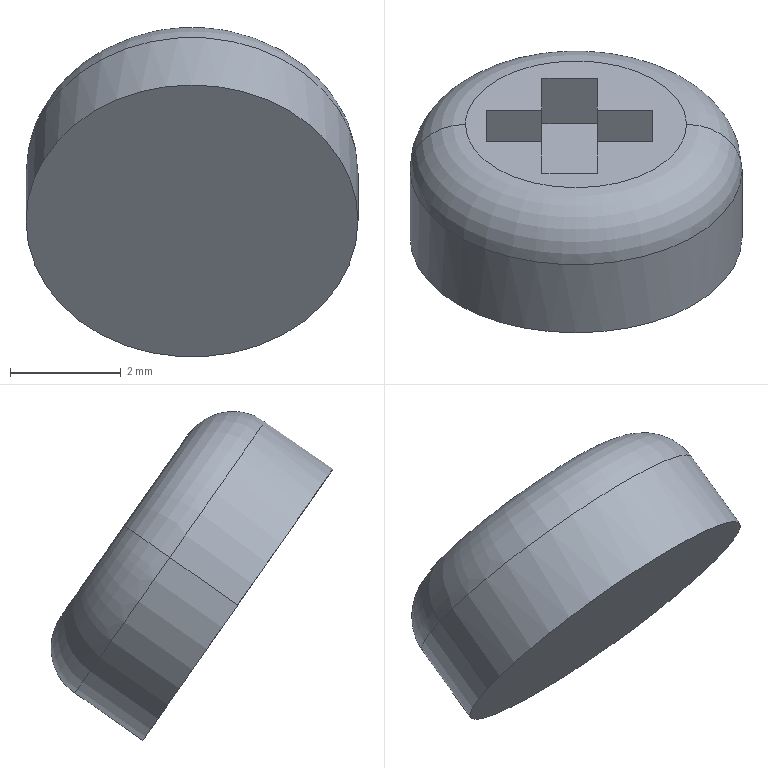Part | STEP file | Positioning_id1730_x_t | 1 solid | 19 faces | box 6 x 5.097 x 5.956 mm | volume 61.942 mm3 | plane 15 | torus 2 | cylinder 2 | commonest cylinder face diameters 6 x2
STEP:
#1=CARTESIAN_POINT('',(0.,0.,0.));
#2=DIRECTION('',(0.,0.,1.));
#3=DIRECTION('',(1.,0.,0.));
#4=AXIS2_PLACEMENT_3D('',#1,#2,#3);
#5=CARTESIAN_POINT('',(-705.532,411.251,418.5));
#6=VERTEX_POINT('',#5);
#7=CARTESIAN_POINT('',(-704.532,411.251,418.5));
#8=VERTEX_POINT('',#7);
#9=CARTESIAN_POINT('',(-705.532,411.251,418.5));
#10=DIRECTION('',(1.,0.,0.));
#11=VECTOR('',#10,1.);
#12=LINE('',#9,#11);
#13=CARTESIAN_POINT('',(-704.532,411.251,418.5));
#14=DIRECTION('',(0.,-0.8192,-0.5736));
#15=DIRECTION('',(-1.,0.,0.));
#16=AXIS2_PLACEMENT_3D('',#13,#14,#15);
#17=PLANE('',#16);
#18=CARTESIAN_POINT('',(1.,0.));
#19=DIRECTION('',(-1.,0.));
#20=VECTOR('',#19,1.);
#21=LINE('',#18,#20);
#22=(GEOMETRIC_REPRESENTATION_CONTEXT(2)PARAMETRIC_REPRESENTATION_CONTEXT()REPRESENTATION_CONTEXT('',''));
#23=DEFINITIONAL_REPRESENTATION('',(#21),#22);
#24=PCURVE('',#17,#23);
#25=CARTESIAN_POINT('',(-705.532,411.251,418.5));
#26=DIRECTION('',(0.,-0.5736,0.8192));
#27=DIRECTION('',(1.,0.,0.));
#28=AXIS2_PLACEMENT_3D('',#25,#26,#27);
#29=PLANE('',#28);
#30=CARTESIAN_POINT('',(0.,0.));
#31=DIRECTION('',(1.,0.));
#32=VECTOR('',#31,1.);
#33=LINE('',#30,#32);
#34=(GEOMETRIC_REPRESENTATION_CONTEXT(2)PARAMETRIC_REPRESENTATION_CONTEXT()REPRESENTATION_CONTEXT('',''));
#35=DEFINITIONAL_REPRESENTATION('',(#33),#34);
#36=PCURVE('',#29,#35);
#37=SURFACE_CURVE('',#12,(#24,#36),.PCURVE_S1.);
#38=EDGE_CURVE('',#6,#8,#37,.T.);
#39=ORIENTED_EDGE('',*,*,#38,.F.);
#40=CARTESIAN_POINT('',(-705.532,411.824,417.681));
#41=VERTEX_POINT('',#40);
#42=CARTESIAN_POINT('',(-705.532,411.824,417.681));
#43=DIRECTION('',(0.,-0.5736,0.8192));
#44=VECTOR('',#43,1.);
#45=LINE('',#42,#44);
#46=CARTESIAN_POINT('',(1.,1.));
#47=DIRECTION('',(0.,-1.));
#48=VECTOR('',#47,1.);
#49=LINE('',#46,#48);
#50=(GEOMETRIC_REPRESENTATION_CONTEXT(2)PARAMETRIC_REPRESENTATION_CONTEXT()REPRESENTATION_CONTEXT('',''));
#51=DEFINITIONAL_REPRESENTATION('',(#49),#50);
#52=PCURVE('',#17,#51);
#53=CARTESIAN_POINT('',(-705.532,411.251,418.5));
#54=DIRECTION('',(-1.,0.,0.));
#55=DIRECTION('',(0.,-0.5736,0.8192));
#56=AXIS2_PLACEMENT_3D('',#53,#54,#55);
#57=PLANE('',#56);
#58=CARTESIAN_POINT('',(-1.,0.));
#59=DIRECTION('',(1.,0.));
#60=VECTOR('',#59,1.);
#61=LINE('',#58,#60);
#62=(GEOMETRIC_REPRESENTATION_CONTEXT(2)PARAMETRIC_REPRESENTATION_CONTEXT()REPRESENTATION_CONTEXT('',''));
#63=DEFINITIONAL_REPRESENTATION('',(#61),#62);
#64=PCURVE('',#57,#63);
#65=SURFACE_CURVE('',#45,(#52,#64),.PCURVE_S1.);
#66=EDGE_CURVE('',#41,#6,#65,.T.);
#67=ORIENTED_EDGE('',*,*,#66,.F.);
#68=CARTESIAN_POINT('',(-706.532,411.824,417.681));
#69=VERTEX_POINT('',#68);
#70=CARTESIAN_POINT('',(-706.532,411.824,417.681));
#71=DIRECTION('',(1.,0.,0.));
#72=VECTOR('',#71,1.);
#73=LINE('',#70,#72);
#74=CARTESIAN_POINT('',(2.,1.));
#75=DIRECTION('',(-1.,0.));
#76=VECTOR('',#75,1.);
#77=LINE('',#74,#76);
#78=(GEOMETRIC_REPRESENTATION_CONTEXT(2)PARAMETRIC_REPRESENTATION_CONTEXT()REPRESENTATION_CONTEXT('',''));
#79=DEFINITIONAL_REPRESENTATION('',(#77),#78);
#80=PCURVE('',#17,#79);
#81=CARTESIAN_POINT('',(-705.532,411.824,417.681));
#82=DIRECTION('',(0.,-0.5736,0.8192));
#83=DIRECTION('',(1.,0.,0.));
#84=AXIS2_PLACEMENT_3D('',#81,#82,#83);
#85=PLANE('',#84);
#86=CARTESIAN_POINT('',(-1.,0.));
#87=DIRECTION('',(1.,0.));
#88=VECTOR('',#87,1.);
#89=LINE('',#86,#88);
#90=(GEOMETRIC_REPRESENTATION_CONTEXT(2)PARAMETRIC_REPRESENTATION_CONTEXT()REPRESENTATION_CONTEXT('',''));
#91=DEFINITIONAL_REPRESENTATION('',(#89),#90);
#92=PCURVE('',#85,#91);
#93=SURFACE_CURVE('',#73,(#80,#92),.PCURVE_S1.);
#94=EDGE_CURVE('',#69,#41,#93,.T.);
#95=ORIENTED_EDGE('',*,*,#94,.F.);
#96=CARTESIAN_POINT('',(-706.532,411.251,418.5));
#97=VERTEX_POINT('',#96);
#98=CARTESIAN_POINT('',(-706.532,411.251,418.5));
#99=DIRECTION('',(0.,0.5736,-0.8192));
#100=VECTOR('',#99,1.);
#101=LINE('',#98,#100);
#102=CARTESIAN_POINT('',(2.,0.));
#103=DIRECTION('',(0.,1.));
#104=VECTOR('',#103,1.);
#105=LINE('',#102,#104);
#106=(GEOMETRIC_REPRESENTATION_CONTEXT(2)PARAMETRIC_REPRESENTATION_CONTEXT()REPRESENTATION_CONTEXT('',''));
#107=DEFINITIONAL_REPRESENTATION('',(#105),#106);
#108=PCURVE('',#17,#107);
#109=CARTESIAN_POINT('',(-706.532,411.824,417.681));
#110=DIRECTION('',(1.,0.,0.));
#111=DIRECTION('',(0.,0.5736,-0.8192));
#112=AXIS2_PLACEMENT_3D('',#109,#110,#111);
#113=PLANE('',#112);
#114=CARTESIAN_POINT('',(-1.,0.));
#115=DIRECTION('',(1.,0.));
#116=VECTOR('',#115,1.);
#117=LINE('',#114,#116);
#118=(GEOMETRIC_REPRESENTATION_CONTEXT(2)PARAMETRIC_REPRESENTATION_CONTEXT()REPRESENTATION_CONTEXT('',''));
#119=DEFINITIONAL_REPRESENTATION('',(#117),#118);
#120=PCURVE('',#113,#119);
#121=SURFACE_CURVE('',#101,(#108,#120),.PCURVE_S1.);
#122=EDGE_CURVE('',#97,#69,#121,.T.);
#123=ORIENTED_EDGE('',*,*,#122,.F.);
#124=CARTESIAN_POINT('',(-707.532,411.251,418.5));
#125=VERTEX_POINT('',#124);
#126=CARTESIAN_POINT('',(-707.532,411.251,418.5));
#127=DIRECTION('',(1.,0.,0.));
#128=VECTOR('',#127,1.);
#129=LINE('',#126,#128);
#130=CARTESIAN_POINT('',(3.,0.));
#131=DIRECTION('',(-1.,0.));
#132=VECTOR('',#131,1.);
#133=LINE('',#130,#132);
#134=(GEOMETRIC_REPRESENTATION_CONTEXT(2)PARAMETRIC_REPRESENTATION_CONTEXT()REPRESENTATION_CONTEXT('',''));
#135=DEFINITIONAL_REPRESENTATION('',(#133),#134);
#136=PCURVE('',#17,#135);
#137=CARTESIAN_POINT('',(-707.532,411.251,418.5));
#138=DIRECTION('',(0.,-0.5736,0.8192));
#139=DIRECTION('',(1.,0.,0.));
#140=AXIS2_PLACEMENT_3D('',#137,#138,#139);
#141=PLANE('',#140);
#142=CARTESIAN_POINT('',(0.,0.));
#143=DIRECTION('',(1.,0.));
#144=VECTOR('',#143,1.);
#145=LINE('',#142,#144);
#146=(GEOMETRIC_REPRESENTATION_CONTEXT(2)PARAMETRIC_REPRESENTATION_CONTEXT()REPRESENTATION_CONTEXT('',''));
#147=DEFINITIONAL_REPRESENTATION('',(#145),#146);
#148=PCURVE('',#141,#147);
#149=SURFACE_CURVE('',#129,(#136,#148),.PCURVE_S1.);
#150=EDGE_CURVE('',#125,#97,#149,.T.);
#151=ORIENTED_EDGE('',*,*,#150,.F.);
#152=CARTESIAN_POINT('',(-707.532,410.677,419.319));
#153=VERTEX_POINT('',#152);
#154=CARTESIAN_POINT('',(-707.532,410.677,419.319));
#155=DIRECTION('',(0.,0.5736,-0.8192));
#156=VECTOR('',#155,1.);
#157=LINE('',#154,#156);
#158=CARTESIAN_POINT('',(3.,-1.));
#159=DIRECTION('',(0.,1.));
#160=VECTOR('',#159,1.);
#161=LINE('',#158,#160);
#162=(GEOMETRIC_REPRESENTATION_CONTEXT(2)PARAMETRIC_REPRESENTATION_CONTEXT()REPRESENTATION_CONTEXT('',''));
#163=DEFINITIONAL_REPRESENTATION('',(#161),#162);
#164=PCURVE('',#17,#163);
#165=CARTESIAN_POINT('',(-707.532,410.677,419.319));
#166=DIRECTION('',(1.,0.,0.));
#167=DIRECTION('',(0.,0.5736,-0.8192));
#168=AXIS2_PLACEMENT_3D('',#165,#166,#167);
#169=PLANE('',#168);
#170=CARTESIAN_POINT('',(0.,0.));
#171=DIRECTION('',(1.,0.));
#172=VECTOR('',#171,1.);
#173=LINE('',#170,#172);
#174=(GEOMETRIC_REPRESENTATION_CONTEXT(2)PARAMETRIC_REPRESENTATION_CONTEXT()REPRESENTATION_CONTEXT('',''));
#175=DEFINITIONAL_REPRESENTATION('',(#173),#174);
#176=PCURVE('',#169,#175);
#177=SURFACE_CURVE('',#157,(#164,#176),.PCURVE_S1.);
#178=EDGE_CURVE('',#153,#125,#177,.T.);
#179=ORIENTED_EDGE('',*,*,#178,.F.);
#180=CARTESIAN_POINT('',(-706.532,410.677,419.319));
#181=VERTEX_POINT('',#180);
#182=CARTESIAN_POINT('',(-706.532,410.677,419.319));
#183=DIRECTION('',(-1.,0.,0.));
#184=VECTOR('',#183,1.);
#185=LINE('',#182,#184);
#186=CARTESIAN_POINT('',(2.,-1.));
#187=DIRECTION('',(1.,0.));
#188=VECTOR('',#187,1.);
#189=LINE('',#186,#188);
#190=(GEOMETRIC_REPRESENTATION_CONTEXT(2)PARAMETRIC_REPRESENTATION_CONTEXT()REPRESENTATION_CONTEXT('',''));
#191=DEFINITIONAL_REPRESENTATION('',(#189),#190);
#192=PCURVE('',#17,#191);
#193=CARTESIAN_POINT('',(-706.532,410.677,419.319));
#194=DIRECTION('',(0.,0.5736,-0.8192));
#195=DIRECTION('',(-1.,0.,0.));
#196=AXIS2_PLACEMENT_3D('',#193,#194,#195);
#197=PLANE('',#196);
#198=CARTESIAN_POINT('',(0.,0.));
#199=DIRECTION('',(1.,0.));
#200=VECTOR('',#199,1.);
#201=LINE('',#198,#200);
#202=(GEOMETRIC_REPRESENTATION_CONTEXT(2)PARAMETRIC_REPRESENTATION_CONTEXT()REPRESENTATION_CONTEXT('',''));
#203=DEFINITIONAL_REPRESENTATION('',(#201),#202);
#204=PCURVE('',#197,#203);
#205=SURFACE_CURVE('',#185,(#192,#204),.PCURVE_S1.);
#206=EDGE_CURVE('',#181,#153,#205,.T.);
#207=ORIENTED_EDGE('',*,*,#206,.F.);
#208=CARTESIAN_POINT('',(-706.532,410.104,420.138));
#209=VERTEX_POINT('',#208);
#210=CARTESIAN_POINT('',(-706.532,410.104,420.138));
#211=DIRECTION('',(0.,0.5736,-0.8192));
#212=VECTOR('',#211,1.);
#213=LINE('',#210,#212);
#214=CARTESIAN_POINT('',(2.,-2.));
#215=DIRECTION('',(0.,1.));
#216=VECTOR('',#215,1.);
#217=LINE('',#214,#216);
#218=(GEOMETRIC_REPRESENTATION_CONTEXT(2)PARAMETRIC_REPRESENTATION_CONTEXT()REPRESENTATION_CONTEXT('',''));
#219=DEFINITIONAL_REPRESENTATION('',(#217),#218);
#220=PCURVE('',#17,#219);
#221=CARTESIAN_POINT('',(-706.532,410.677,419.319));
#222=DIRECTION('',(1.,0.,0.));
#223=DIRECTION('',(0.,0.5736,-0.8192));
#224=AXIS2_PLACEMENT_3D('',#221,#222,#223);
#225=PLANE('',#224);
#226=CARTESIAN_POINT('',(-1.,0.));
#227=DIRECTION('',(1.,0.));
#228=VECTOR('',#227,1.);
#229=LINE('',#226,#228);
#230=(GEOMETRIC_REPRESENTATION_CONTEXT(2)PARAMETRIC_REPRESENTATION_CONTEXT()REPRESENTATION_CONTEXT('',''));
#231=DEFINITIONAL_REPRESENTATION('',(#229),#230);
#232=PCURVE('',#225,#231);
#233=SURFACE_CURVE('',#213,(#220,#232),.PCURVE_S1.);
#234=EDGE_CURVE('',#209,#181,#233,.T.);
#235=ORIENTED_EDGE('',*,*,#234,.F.);
#236=CARTESIAN_POINT('',(-705.532,410.104,420.138));
#237=VERTEX_POINT('',#236);
#238=CARTESIAN_POINT('',(-705.532,410.104,420.138));
#239=DIRECTION('',(-1.,0.,0.));
#240=VECTOR('',#239,1.);
#241=LINE('',#238,#240);
#242=CARTESIAN_POINT('',(1.,-2.));
#243=DIRECTION('',(1.,0.));
#244=VECTOR('',#243,1.);
#245=LINE('',#242,#244);
#246=(GEOMETRIC_REPRESENTATION_CONTEXT(2)PARAMETRIC_REPRESENTATION_CONTEXT()REPRESENTATION_CONTEXT('',''));
#247=DEFINITIONAL_REPRESENTATION('',(#245),#246);
#248=PCURVE('',#17,#247);
#249=CARTESIAN_POINT('',(-706.532,410.104,420.138));
#250=DIRECTION('',(0.,0.5736,-0.8192));
#251=DIRECTION('',(-1.,0.,0.));
#252=AXIS2_PLACEMENT_3D('',#249,#250,#251);
#253=PLANE('',#252);
#254=CARTESIAN_POINT('',(-1.,0.));
#255=DIRECTION('',(1.,0.));
#256=VECTOR('',#255,1.);
#257=LINE('',#254,#256);
#258=(GEOMETRIC_REPRESENTATION_CONTEXT(2)PARAMETRIC_REPRESENTATION_CONTEXT()REPRESENTATION_CONTEXT('',''));
#259=DEFINITIONAL_REPRESENTATION('',(#257),#258);
#260=PCURVE('',#253,#259);
#261=SURFACE_CURVE('',#241,(#248,#260),.PCURVE_S1.);
#262=EDGE_CURVE('',#237,#209,#261,.T.);
#263=ORIENTED_EDGE('',*,*,#262,.F.);
#264=CARTESIAN_POINT('',(-705.532,410.677,419.319));
#265=VERTEX_POINT('',#264);
#266=CARTESIAN_POINT('',(-705.532,410.677,419.319));
#267=DIRECTION('',(0.,-0.5736,0.8192));
#268=VECTOR('',#267,1.);
#269=LINE('',#266,#268);
#270=CARTESIAN_POINT('',(1.,-1.));
#271=DIRECTION('',(0.,-1.));
#272=VECTOR('',#271,1.);
#273=LINE('',#270,#272);
#274=(GEOMETRIC_REPRESENTATION_CONTEXT(2)PARAMETRIC_REPRESENTATION_CONTEXT()REPRESENTATION_CONTEXT('',''));
#275=DEFINITIONAL_REPRESENTATION('',(#273),#274);
#276=PCURVE('',#17,#275);
#277=CARTESIAN_POINT('',(-705.532,410.104,420.138));
#278=DIRECTION('',(-1.,0.,0.));
#279=DIRECTION('',(0.,-0.5736,0.8192));
#280=AXIS2_PLACEMENT_3D('',#277,#278,#279);
#281=PLANE('',#280);
#282=CARTESIAN_POINT('',(-1.,0.));
#283=DIRECTION('',(1.,0.));
#284=VECTOR('',#283,1.);
#285=LINE('',#282,#284);
#286=(GEOMETRIC_REPRESENTATION_CONTEXT(2)PARAMETRIC_REPRESENTATION_CONTEXT()REPRESENTATION_CONTEXT('',''));
#287=DEFINITIONAL_REPRESENTATION('',(#285),#286);
#288=PCURVE('',#281,#287);
#289=SURFACE_CURVE('',#269,(#276,#288),.PCURVE_S1.);
#290=EDGE_CURVE('',#265,#237,#289,.T.);
#291=ORIENTED_EDGE('',*,*,#290,.F.);
#292=CARTESIAN_POINT('',(-704.532,410.677,419.319));
#293=VERTEX_POINT('',#292);
#294=CARTESIAN_POINT('',(-704.532,410.677,419.319));
#295=DIRECTION('',(-1.,0.,0.));
#296=VECTOR('',#295,1.);
#297=LINE('',#294,#296);
#298=CARTESIAN_POINT('',(0.,-1.));
#299=DIRECTION('',(1.,0.));
#300=VECTOR('',#299,1.);
#301=LINE('',#298,#300);
#302=(GEOMETRIC_REPRESENTATION_CONTEXT(2)PARAMETRIC_REPRESENTATION_CONTEXT()REPRESENTATION_CONTEXT('',''));
#303=DEFINITIONAL_REPRESENTATION('',(#301),#302);
#304=PCURVE('',#17,#303);
#305=CARTESIAN_POINT('',(-704.532,410.677,419.319));
#306=DIRECTION('',(0.,0.5736,-0.8192));
#307=DIRECTION('',(-1.,0.,0.));
#308=AXIS2_PLACEMENT_3D('',#305,#306,#307);
#309=PLANE('',#308);
#310=CARTESIAN_POINT('',(0.,0.));
#311=DIRECTION('',(1.,0.));
#312=VECTOR('',#311,1.);
#313=LINE('',#310,#312);
#314=(GEOMETRIC_REPRESENTATION_CONTEXT(2)PARAMETRIC_REPRESENTATION_CONTEXT()REPRESENTATION_CONTEXT('',''));
#315=DEFINITIONAL_REPRESENTATION('',(#313),#314);
#316=PCURVE('',#309,#315);
#317=SURFACE_CURVE('',#297,(#304,#316),.PCURVE_S1.);
#318=EDGE_CURVE('',#293,#265,#317,.T.);
#319=ORIENTED_EDGE('',*,*,#318,.F.);
#320=CARTESIAN_POINT('',(-704.532,411.251,418.5));
#321=DIRECTION('',(0.,-0.5736,0.8192));
#322=VECTOR('',#321,1.);
#323=LINE('',#320,#322);
#324=CARTESIAN_POINT('',(0.,0.));
#325=DIRECTION('',(0.,-1.));
#326=VECTOR('',#325,1.);
#327=LINE('',#324,#326);
#328=(GEOMETRIC_REPRESENTATION_CONTEXT(2)PARAMETRIC_REPRESENTATION_CONTEXT()REPRESENTATION_CONTEXT('',''));
#329=DEFINITIONAL_REPRESENTATION('',(#327),#328);
#330=PCURVE('',#17,#329);
#331=CARTESIAN_POINT('',(-704.532,411.251,418.5));
#332=DIRECTION('',(-1.,0.,0.));
#333=DIRECTION('',(0.,-0.5736,0.8192));
#334=AXIS2_PLACEMENT_3D('',#331,#332,#333);
#335=PLANE('',#334);
#336=CARTESIAN_POINT('',(0.,0.));
#337=DIRECTION('',(1.,0.));
#338=VECTOR('',#337,1.);
#339=LINE('',#336,#338);
#340=(GEOMETRIC_REPRESENTATION_CONTEXT(2)PARAMETRIC_REPRESENTATION_CONTEXT()REPRESENTATION_CONTEXT('',''));
#341=DEFINITIONAL_REPRESENTATION('',(#339),#340);
#342=PCURVE('',#335,#341);
#343=SURFACE_CURVE('',#323,(#330,#342),.PCURVE_S1.);
#344=EDGE_CURVE('',#8,#293,#343,.T.);
#345=ORIENTED_EDGE('',*,*,#344,.F.);
#346=EDGE_LOOP('',(#39,#67,#95,#123,#151,#179,#207,#235,#263,#291,#319,#345));
#347=FACE_BOUND('',#346,.T.);
#348=ADVANCED_FACE('',(#347),#17,.F.);
#349=ORIENTED_EDGE('',*,*,#66,.T.);
#350=CARTESIAN_POINT('',(-705.532,412.07,419.074));
#351=VERTEX_POINT('',#350);
#352=CARTESIAN_POINT('',(-705.532,411.251,418.5));
#353=DIRECTION('',(0.,0.8192,0.5736));
#354=VECTOR('',#353,1.);
#355=LINE('',#352,#354);
#356=CARTESIAN_POINT('',(0.,0.));
#357=DIRECTION('',(0.,1.));
#358=VECTOR('',#357,1.);
#359=LINE('',#356,#358);
#360=(GEOMETRIC_REPRESENTATION_CONTEXT(2)PARAMETRIC_REPRESENTATION_CONTEXT()REPRESENTATION_CONTEXT('',''));
#361=DEFINITIONAL_REPRESENTATION('',(#359),#360);
#362=PCURVE('',#57,#361);
#363=CARTESIAN_POINT('',(0.,0.));
#364=DIRECTION('',(0.,1.));
#365=VECTOR('',#364,1.);
#366=LINE('',#363,#365);
#367=(GEOMETRIC_REPRESENTATION_CONTEXT(2)PARAMETRIC_REPRESENTATION_CONTEXT()REPRESENTATION_CONTEXT('',''));
#368=DEFINITIONAL_REPRESENTATION('',(#366),#367);
#369=PCURVE('',#29,#368);
#370=SURFACE_CURVE('',#355,(#362,#369),.PCURVE_S1.);
#371=EDGE_CURVE('',#6,#351,#370,.T.);
#372=ORIENTED_EDGE('',*,*,#371,.T.);
#373=CARTESIAN_POINT('',(-705.532,412.644,418.255));
#374=VERTEX_POINT('',#373);
#375=CARTESIAN_POINT('',(-705.532,412.644,418.255));
#376=DIRECTION('',(0.,-0.5736,0.8192));
#377=VECTOR('',#376,1.);
#378=LINE('',#375,#377);
#379=CARTESIAN_POINT('',(-1.,1.));
#380=DIRECTION('',(1.,0.));
#381=VECTOR('',#380,1.);
#382=LINE('',#379,#381);
#383=(GEOMETRIC_REPRESENTATION_CONTEXT(2)PARAMETRIC_REPRESENTATION_CONTEXT()REPRESENTATION_CONTEXT('',''));
#384=DEFINITIONAL_REPRESENTATION('',(#382),#383);
#385=PCURVE('',#57,#384);
#386=CARTESIAN_POINT('',(-705.916,411.811,419.444));
#387=DIRECTION('',(0.,-0.8192,-0.5736));
#388=DIRECTION('',(-1.,0.,0.));
#389=AXIS2_PLACEMENT_3D('',#386,#387,#388);
#390=PLANE('',#389);
#391=CARTESIAN_POINT('',(-0.3848,1.452));
#392=DIRECTION('',(0.,-1.));
#393=VECTOR('',#392,1.);
#394=LINE('',#391,#393);
#395=(GEOMETRIC_REPRESENTATION_CONTEXT(2)PARAMETRIC_REPRESENTATION_CONTEXT()REPRESENTATION_CONTEXT('',''));
#396=DEFINITIONAL_REPRESENTATION('',(#394),#395);
#397=PCURVE('',#390,#396);
#398=SURFACE_CURVE('',#378,(#385,#397),.PCURVE_S1.);
#399=EDGE_CURVE('',#374,#351,#398,.T.);
#400=ORIENTED_EDGE('',*,*,#399,.F.);
#401=CARTESIAN_POINT('',(-705.532,411.824,417.681));
#402=DIRECTION('',(0.,0.8192,0.5736));
#403=VECTOR('',#402,1.);
#404=LINE('',#401,#403);
#405=CARTESIAN_POINT('',(-1.,0.));
#406=DIRECTION('',(0.,1.));
#407=VECTOR('',#406,1.);
#408=LINE('',#405,#407);
#409=(GEOMETRIC_REPRESENTATION_CONTEXT(2)PARAMETRIC_REPRESENTATION_CONTEXT()REPRESENTATION_CONTEXT('',''));
#410=DEFINITIONAL_REPRESENTATION('',(#408),#409);
#411=PCURVE('',#57,#410);
#412=CARTESIAN_POINT('',(0.,0.));
#413=DIRECTION('',(0.,1.));
#414=VECTOR('',#413,1.);
#415=LINE('',#412,#414);
#416=(GEOMETRIC_REPRESENTATION_CONTEXT(2)PARAMETRIC_REPRESENTATION_CONTEXT()REPRESENTATION_CONTEXT('',''));
#417=DEFINITIONAL_REPRESENTATION('',(#415),#416);
#418=PCURVE('',#85,#417);
#419=SURFACE_CURVE('',#404,(#411,#418),.PCURVE_S1.);
#420=EDGE_CURVE('',#41,#374,#419,.T.);
#421=ORIENTED_EDGE('',*,*,#420,.F.);
#422=EDGE_LOOP('',(#349,#372,#400,#421));
#423=FACE_BOUND('',#422,.T.);
#424=ADVANCED_FACE('',(#423),#57,.T.);
#425=ORIENTED_EDGE('',*,*,#420,.T.);
#426=CARTESIAN_POINT('',(-706.532,412.644,418.255));
#427=VERTEX_POINT('',#426);
#428=CARTESIAN_POINT('',(-706.532,412.644,418.255));
#429=DIRECTION('',(1.,0.,0.));
#430=VECTOR('',#429,1.);
#431=LINE('',#428,#430);
#432=CARTESIAN_POINT('',(-1.,1.));
#433=DIRECTION('',(1.,0.));
#434=VECTOR('',#433,1.);
#435=LINE('',#432,#434);
#436=(GEOMETRIC_REPRESENTATION_CONTEXT(2)PARAMETRIC_REPRESENTATION_CONTEXT()REPRESENTATION_CONTEXT('',''));
#437=DEFINITIONAL_REPRESENTATION('',(#435),#436);
#438=PCURVE('',#85,#437);
#439=CARTESIAN_POINT('',(0.6152,1.452));
#440=DIRECTION('',(-1.,0.));
#441=VECTOR('',#440,1.);
#442=LINE('',#439,#441);
#443=(GEOMETRIC_REPRESENTATION_CONTEXT(2)PARAMETRIC_REPRESENTATION_CONTEXT()REPRESENTATION_CONTEXT('',''));
#444=DEFINITIONAL_REPRESENTATION('',(#442),#443);
#445=PCURVE('',#390,#444);
#446=SURFACE_CURVE('',#431,(#438,#445),.PCURVE_S1.);
#447=EDGE_CURVE('',#427,#374,#446,.T.);
#448=ORIENTED_EDGE('',*,*,#447,.F.);
#449=CARTESIAN_POINT('',(-706.532,411.824,417.681));
#450=DIRECTION('',(0.,0.8192,0.5736));
#451=VECTOR('',#450,1.);
#452=LINE('',#449,#451);
#453=CARTESIAN_POINT('',(-1.,0.));
#454=DIRECTION('',(0.,1.));
#455=VECTOR('',#454,1.);
#456=LINE('',#453,#455);
#457=(GEOMETRIC_REPRESENTATION_CONTEXT(2)PARAMETRIC_REPRESENTATION_CONTEXT()REPRESENTATION_CONTEXT('',''));
#458=DEFINITIONAL_REPRESENTATION('',(#456),#457);
#459=PCURVE('',#85,#458);
#460=CARTESIAN_POINT('',(0.,0.));
#461=DIRECTION('',(0.,1.));
#462=VECTOR('',#461,1.);
#463=LINE('',#460,#462);
#464=(GEOMETRIC_REPRESENTATION_CONTEXT(2)PARAMETRIC_REPRESENTATION_CONTEXT()REPRESENTATION_CONTEXT('',''));
#465=DEFINITIONAL_REPRESENTATION('',(#463),#464);
#466=PCURVE('',#113,#465);
#467=SURFACE_CURVE('',#452,(#459,#466),.PCURVE_S1.);
#468=EDGE_CURVE('',#69,#427,#467,.T.);
#469=ORIENTED_EDGE('',*,*,#468,.F.);
#470=ORIENTED_EDGE('',*,*,#94,.T.);
#471=EDGE_LOOP('',(#425,#448,#469,#470));
#472=FACE_BOUND('',#471,.T.);
#473=ADVANCED_FACE('',(#472),#85,.T.);
#474=ORIENTED_EDGE('',*,*,#468,.T.);
#475=CARTESIAN_POINT('',(-706.532,412.07,419.074));
#476=VERTEX_POINT('',#475);
#477=CARTESIAN_POINT('',(-706.532,412.07,419.074));
#478=DIRECTION('',(0.,0.5736,-0.8192));
#479=VECTOR('',#478,1.);
#480=LINE('',#477,#479);
#481=CARTESIAN_POINT('',(-1.,1.));
#482=DIRECTION('',(1.,0.));
#483=VECTOR('',#482,1.);
#484=LINE('',#481,#483);
#485=(GEOMETRIC_REPRESENTATION_CONTEXT(2)PARAMETRIC_REPRESENTATION_CONTEXT()REPRESENTATION_CONTEXT('',''));
#486=DEFINITIONAL_REPRESENTATION('',(#484),#485);
#487=PCURVE('',#113,#486);
#488=CARTESIAN_POINT('',(0.6152,0.4516));
#489=DIRECTION('',(0.,1.));
#490=VECTOR('',#489,1.);
#491=LINE('',#488,#490);
#492=(GEOMETRIC_REPRESENTATION_CONTEXT(2)PARAMETRIC_REPRESENTATION_CONTEXT()REPRESENTATION_CONTEXT('',''));
#493=DEFINITIONAL_REPRESENTATION('',(#491),#492);
#494=PCURVE('',#390,#493);
#495=SURFACE_CURVE('',#480,(#487,#494),.PCURVE_S1.);
#496=EDGE_CURVE('',#476,#427,#495,.T.);
#497=ORIENTED_EDGE('',*,*,#496,.F.);
#498=CARTESIAN_POINT('',(-706.532,411.251,418.5));
#499=DIRECTION('',(0.,0.8192,0.5736));
#500=VECTOR('',#499,1.);
#501=LINE('',#498,#500);
#502=CARTESIAN_POINT('',(-1.,0.));
#503=DIRECTION('',(0.,1.));
#504=VECTOR('',#503,1.);
#505=LINE('',#502,#504);
#506=(GEOMETRIC_REPRESENTATION_CONTEXT(2)PARAMETRIC_REPRESENTATION_CONTEXT()REPRESENTATION_CONTEXT('',''));
#507=DEFINITIONAL_REPRESENTATION('',(#505),#506);
#508=PCURVE('',#113,#507);
#509=CARTESIAN_POINT('',(1.,0.));
#510=DIRECTION('',(0.,1.));
#511=VECTOR('',#510,1.);
#512=LINE('',#509,#511);
#513=(GEOMETRIC_REPRESENTATION_CONTEXT(2)PARAMETRIC_REPRESENTATION_CONTEXT()REPRESENTATION_CONTEXT('',''));
#514=DEFINITIONAL_REPRESENTATION('',(#512),#513);
#515=PCURVE('',#141,#514);
#516=SURFACE_CURVE('',#501,(#508,#515),.PCURVE_S1.);
#517=EDGE_CURVE('',#97,#476,#516,.T.);
#518=ORIENTED_EDGE('',*,*,#517,.F.);
#519=ORIENTED_EDGE('',*,*,#122,.T.);
#520=EDGE_LOOP('',(#474,#497,#518,#519));
#521=FACE_BOUND('',#520,.T.);
#522=ADVANCED_FACE('',(#521),#113,.T.);
#523=ORIENTED_EDGE('',*,*,#517,.T.);
#524=CARTESIAN_POINT('',(-707.532,412.07,419.074));
#525=VERTEX_POINT('',#524);
#526=CARTESIAN_POINT('',(-707.532,412.07,419.074));
#527=DIRECTION('',(1.,0.,0.));
#528=VECTOR('',#527,1.);
#529=LINE('',#526,#528);
#530=CARTESIAN_POINT('',(0.,1.));
#531=DIRECTION('',(1.,0.));
#532=VECTOR('',#531,1.);
#533=LINE('',#530,#532);
#534=(GEOMETRIC_REPRESENTATION_CONTEXT(2)PARAMETRIC_REPRESENTATION_CONTEXT()REPRESENTATION_CONTEXT('',''));
#535=DEFINITIONAL_REPRESENTATION('',(#533),#534);
#536=PCURVE('',#141,#535);
#537=CARTESIAN_POINT('',(1.615,0.4516));
#538=DIRECTION('',(-1.,0.));
#539=VECTOR('',#538,1.);
#540=LINE('',#537,#539);
#541=(GEOMETRIC_REPRESENTATION_CONTEXT(2)PARAMETRIC_REPRESENTATION_CONTEXT()REPRESENTATION_CONTEXT('',''));
#542=DEFINITIONAL_REPRESENTATION('',(#540),#541);
#543=PCURVE('',#390,#542);
#544=SURFACE_CURVE('',#529,(#536,#543),.PCURVE_S1.);
#545=EDGE_CURVE('',#525,#476,#544,.T.);
#546=ORIENTED_EDGE('',*,*,#545,.F.);
#547=CARTESIAN_POINT('',(-707.532,411.251,418.5));
#548=DIRECTION('',(0.,0.8192,0.5736));
#549=VECTOR('',#548,1.);
#550=LINE('',#547,#549);
#551=CARTESIAN_POINT('',(0.,0.));
#552=DIRECTION('',(0.,1.));
#553=VECTOR('',#552,1.);
#554=LINE('',#551,#553);
#555=(GEOMETRIC_REPRESENTATION_CONTEXT(2)PARAMETRIC_REPRESENTATION_CONTEXT()REPRESENTATION_CONTEXT('',''));
#556=DEFINITIONAL_REPRESENTATION('',(#554),#555);
#557=PCURVE('',#141,#556);
#558=CARTESIAN_POINT('',(1.,0.));
#559=DIRECTION('',(0.,1.));
#560=VECTOR('',#559,1.);
#561=LINE('',#558,#560);
#562=(GEOMETRIC_REPRESENTATION_CONTEXT(2)PARAMETRIC_REPRESENTATION_CONTEXT()REPRESENTATION_CONTEXT('',''));
#563=DEFINITIONAL_REPRESENTATION('',(#561),#562);
#564=PCURVE('',#169,#563);
#565=SURFACE_CURVE('',#550,(#557,#564),.PCURVE_S1.);
#566=EDGE_CURVE('',#125,#525,#565,.T.);
#567=ORIENTED_EDGE('',*,*,#566,.F.);
#568=ORIENTED_EDGE('',*,*,#150,.T.);
#569=EDGE_LOOP('',(#523,#546,#567,#568));
#570=FACE_BOUND('',#569,.T.);
#571=ADVANCED_FACE('',(#570),#141,.T.);
#572=ORIENTED_EDGE('',*,*,#566,.T.);
#573=CARTESIAN_POINT('',(-707.532,411.496,419.893));
#574=VERTEX_POINT('',#573);
#575=CARTESIAN_POINT('',(-707.532,411.496,419.893));
#576=DIRECTION('',(0.,0.5736,-0.8192));
#577=VECTOR('',#576,1.);
#578=LINE('',#575,#577);
#579=CARTESIAN_POINT('',(0.,1.));
#580=DIRECTION('',(1.,0.));
#581=VECTOR('',#580,1.);
#582=LINE('',#579,#581);
#583=(GEOMETRIC_REPRESENTATION_CONTEXT(2)PARAMETRIC_REPRESENTATION_CONTEXT()REPRESENTATION_CONTEXT('',''));
#584=DEFINITIONAL_REPRESENTATION('',(#582),#583);
#585=PCURVE('',#169,#584);
#586=CARTESIAN_POINT('',(1.615,-0.5484));
#587=DIRECTION('',(0.,1.));
#588=VECTOR('',#587,1.);
#589=LINE('',#586,#588);
#590=(GEOMETRIC_REPRESENTATION_CONTEXT(2)PARAMETRIC_REPRESENTATION_CONTEXT()REPRESENTATION_CONTEXT('',''));
#591=DEFINITIONAL_REPRESENTATION('',(#589),#590);
#592=PCURVE('',#390,#591);
#593=SURFACE_CURVE('',#578,(#585,#592),.PCURVE_S1.);
#594=EDGE_CURVE('',#574,#525,#593,.T.);
#595=ORIENTED_EDGE('',*,*,#594,.F.);
#596=CARTESIAN_POINT('',(-707.532,410.677,419.319));
#597=DIRECTION('',(0.,0.8192,0.5736));
#598=VECTOR('',#597,1.);
#599=LINE('',#596,#598);
#600=CARTESIAN_POINT('',(0.,0.));
#601=DIRECTION('',(0.,1.));
#602=VECTOR('',#601,1.);
#603=LINE('',#600,#602);
#604=(GEOMETRIC_REPRESENTATION_CONTEXT(2)PARAMETRIC_REPRESENTATION_CONTEXT()REPRESENTATION_CONTEXT('',''));
#605=DEFINITIONAL_REPRESENTATION('',(#603),#604);
#606=PCURVE('',#169,#605);
#607=CARTESIAN_POINT('',(1.,0.));
#608=DIRECTION('',(0.,1.));
#609=VECTOR('',#608,1.);
#610=LINE('',#607,#609);
#611=(GEOMETRIC_REPRESENTATION_CONTEXT(2)PARAMETRIC_REPRESENTATION_CONTEXT()REPRESENTATION_CONTEXT('',''));
#612=DEFINITIONAL_REPRESENTATION('',(#610),#611);
#613=PCURVE('',#197,#612);
#614=SURFACE_CURVE('',#599,(#606,#613),.PCURVE_S1.);
#615=EDGE_CURVE('',#153,#574,#614,.T.);
#616=ORIENTED_EDGE('',*,*,#615,.F.);
#617=ORIENTED_EDGE('',*,*,#178,.T.);
#618=EDGE_LOOP('',(#572,#595,#616,#617));
#619=FACE_BOUND('',#618,.T.);
#620=ADVANCED_FACE('',(#619),#169,.T.);
#621=ORIENTED_EDGE('',*,*,#615,.T.);
#622=CARTESIAN_POINT('',(-706.532,411.496,419.893));
#623=VERTEX_POINT('',#622);
#624=CARTESIAN_POINT('',(-706.532,411.496,419.893));
#625=DIRECTION('',(-1.,0.,0.));
#626=VECTOR('',#625,1.);
#627=LINE('',#624,#626);
#628=CARTESIAN_POINT('',(0.,1.));
#629=DIRECTION('',(1.,0.));
#630=VECTOR('',#629,1.);
#631=LINE('',#628,#630);
#632=(GEOMETRIC_REPRESENTATION_CONTEXT(2)PARAMETRIC_REPRESENTATION_CONTEXT()REPRESENTATION_CONTEXT('',''));
#633=DEFINITIONAL_REPRESENTATION('',(#631),#632);
#634=PCURVE('',#197,#633);
#635=CARTESIAN_POINT('',(0.6152,-0.5484));
#636=DIRECTION('',(1.,0.));
#637=VECTOR('',#636,1.);
#638=LINE('',#635,#637);
#639=(GEOMETRIC_REPRESENTATION_CONTEXT(2)PARAMETRIC_REPRESENTATION_CONTEXT()REPRESENTATION_CONTEXT('',''));
#640=DEFINITIONAL_REPRESENTATION('',(#638),#639);
#641=PCURVE('',#390,#640);
#642=SURFACE_CURVE('',#627,(#634,#641),.PCURVE_S1.);
#643=EDGE_CURVE('',#623,#574,#642,.T.);
#644=ORIENTED_EDGE('',*,*,#643,.F.);
#645=CARTESIAN_POINT('',(-706.532,410.677,419.319));
#646=DIRECTION('',(0.,0.8192,0.5736));
#647=VECTOR('',#646,1.);
#648=LINE('',#645,#647);
#649=CARTESIAN_POINT('',(0.,0.));
#650=DIRECTION('',(0.,1.));
#651=VECTOR('',#650,1.);
#652=LINE('',#649,#651);
#653=(GEOMETRIC_REPRESENTATION_CONTEXT(2)PARAMETRIC_REPRESENTATION_CONTEXT()REPRESENTATION_CONTEXT('',''));
#654=DEFINITIONAL_REPRESENTATION('',(#652),#653);
#655=PCURVE('',#197,#654);
#656=CARTESIAN_POINT('',(0.,0.));
#657=DIRECTION('',(0.,1.));
#658=VECTOR('',#657,1.);
#659=LINE('',#656,#658);
#660=(GEOMETRIC_REPRESENTATION_CONTEXT(2)PARAMETRIC_REPRESENTATION_CONTEXT()REPRESENTATION_CONTEXT('',''));
#661=DEFINITIONAL_REPRESENTATION('',(#659),#660);
#662=PCURVE('',#225,#661);
#663=SURFACE_CURVE('',#648,(#655,#662),.PCURVE_S1.);
#664=EDGE_CURVE('',#181,#623,#663,.T.);
#665=ORIENTED_EDGE('',*,*,#664,.F.);
#666=ORIENTED_EDGE('',*,*,#206,.T.);
#667=EDGE_LOOP('',(#621,#644,#665,#666));
#668=FACE_BOUND('',#667,.T.);
#669=ADVANCED_FACE('',(#668),#197,.T.);
#670=ORIENTED_EDGE('',*,*,#664,.T.);
#671=CARTESIAN_POINT('',(-706.532,410.923,420.712));
#672=VERTEX_POINT('',#671);
#673=CARTESIAN_POINT('',(-706.532,410.923,420.712));
#674=DIRECTION('',(0.,0.5736,-0.8192));
#675=VECTOR('',#674,1.);
#676=LINE('',#673,#675);
#677=CARTESIAN_POINT('',(-1.,1.));
#678=DIRECTION('',(1.,0.));
#679=VECTOR('',#678,1.);
#680=LINE('',#677,#679);
#681=(GEOMETRIC_REPRESENTATION_CONTEXT(2)PARAMETRIC_REPRESENTATION_CONTEXT()REPRESENTATION_CONTEXT('',''));
#682=DEFINITIONAL_REPRESENTATION('',(#680),#681);
#683=PCURVE('',#225,#682);
#684=CARTESIAN_POINT('',(0.6152,-1.548));
#685=DIRECTION('',(0.,1.));
#686=VECTOR('',#685,1.);
#687=LINE('',#684,#686);
#688=(GEOMETRIC_REPRESENTATION_CONTEXT(2)PARAMETRIC_REPRESENTATION_CONTEXT()REPRESENTATION_CONTEXT('',''));
#689=DEFINITIONAL_REPRESENTATION('',(#687),#688);
#690=PCURVE('',#390,#689);
#691=SURFACE_CURVE('',#676,(#683,#690),.PCURVE_S1.);
#692=EDGE_CURVE('',#672,#623,#691,.T.);
#693=ORIENTED_EDGE('',*,*,#692,.F.);
#694=CARTESIAN_POINT('',(-706.532,410.104,420.138));
#695=DIRECTION('',(0.,0.8192,0.5736));
#696=VECTOR('',#695,1.);
#697=LINE('',#694,#696);
#698=CARTESIAN_POINT('',(-1.,0.));
#699=DIRECTION('',(0.,1.));
#700=VECTOR('',#699,1.);
#701=LINE('',#698,#700);
#702=(GEOMETRIC_REPRESENTATION_CONTEXT(2)PARAMETRIC_REPRESENTATION_CONTEXT()REPRESENTATION_CONTEXT('',''));
#703=DEFINITIONAL_REPRESENTATION('',(#701),#702);
#704=PCURVE('',#225,#703);
#705=CARTESIAN_POINT('',(0.,0.));
#706=DIRECTION('',(0.,1.));
#707=VECTOR('',#706,1.);
#708=LINE('',#705,#707);
#709=(GEOMETRIC_REPRESENTATION_CONTEXT(2)PARAMETRIC_REPRESENTATION_CONTEXT()REPRESENTATION_CONTEXT('',''));
#710=DEFINITIONAL_REPRESENTATION('',(#708),#709);
#711=PCURVE('',#253,#710);
#712=SURFACE_CURVE('',#697,(#704,#711),.PCURVE_S1.);
#713=EDGE_CURVE('',#209,#672,#712,.T.);
#714=ORIENTED_EDGE('',*,*,#713,.F.);
#715=ORIENTED_EDGE('',*,*,#234,.T.);
#716=EDGE_LOOP('',(#670,#693,#714,#715));
#717=FACE_BOUND('',#716,.T.);
#718=ADVANCED_FACE('',(#717),#225,.T.);
#719=ORIENTED_EDGE('',*,*,#713,.T.);
#720=CARTESIAN_POINT('',(-705.532,410.923,420.712));
#721=VERTEX_POINT('',#720);
#722=CARTESIAN_POINT('',(-705.532,410.923,420.712));
#723=DIRECTION('',(-1.,0.,0.));
#724=VECTOR('',#723,1.);
#725=LINE('',#722,#724);
#726=CARTESIAN_POINT('',(-1.,1.));
#727=DIRECTION('',(1.,0.));
#728=VECTOR('',#727,1.);
#729=LINE('',#726,#728);
#730=(GEOMETRIC_REPRESENTATION_CONTEXT(2)PARAMETRIC_REPRESENTATION_CONTEXT()REPRESENTATION_CONTEXT('',''));
#731=DEFINITIONAL_REPRESENTATION('',(#729),#730);
#732=PCURVE('',#253,#731);
#733=CARTESIAN_POINT('',(-0.3848,-1.548));
#734=DIRECTION('',(1.,0.));
#735=VECTOR('',#734,1.);
#736=LINE('',#733,#735);
#737=(GEOMETRIC_REPRESENTATION_CONTEXT(2)PARAMETRIC_REPRESENTATION_CONTEXT()REPRESENTATION_CONTEXT('',''));
#738=DEFINITIONAL_REPRESENTATION('',(#736),#737);
#739=PCURVE('',#390,#738);
#740=SURFACE_CURVE('',#725,(#732,#739),.PCURVE_S1.);
#741=EDGE_CURVE('',#721,#672,#740,.T.);
#742=ORIENTED_EDGE('',*,*,#741,.F.);
#743=CARTESIAN_POINT('',(-705.532,410.104,420.138));
#744=DIRECTION('',(0.,0.8192,0.5736));
#745=VECTOR('',#744,1.);
#746=LINE('',#743,#745);
#747=CARTESIAN_POINT('',(-1.,0.));
#748=DIRECTION('',(0.,1.));
#749=VECTOR('',#748,1.);
#750=LINE('',#747,#749);
#751=(GEOMETRIC_REPRESENTATION_CONTEXT(2)PARAMETRIC_REPRESENTATION_CONTEXT()REPRESENTATION_CONTEXT('',''));
#752=DEFINITIONAL_REPRESENTATION('',(#750),#751);
#753=PCURVE('',#253,#752);
#754=CARTESIAN_POINT('',(0.,0.));
#755=DIRECTION('',(0.,1.));
#756=VECTOR('',#755,1.);
#757=LINE('',#754,#756);
#758=(GEOMETRIC_REPRESENTATION_CONTEXT(2)PARAMETRIC_REPRESENTATION_CONTEXT()REPRESENTATION_CONTEXT('',''));
#759=DEFINITIONAL_REPRESENTATION('',(#757),#758);
#760=PCURVE('',#281,#759);
#761=SURFACE_CURVE('',#746,(#753,#760),.PCURVE_S1.);
#762=EDGE_CURVE('',#237,#721,#761,.T.);
#763=ORIENTED_EDGE('',*,*,#762,.F.);
#764=ORIENTED_EDGE('',*,*,#262,.T.);
#765=EDGE_LOOP('',(#719,#742,#763,#764));
#766=FACE_BOUND('',#765,.T.);
#767=ADVANCED_FACE('',(#766),#253,.T.);
#768=ORIENTED_EDGE('',*,*,#762,.T.);
#769=CARTESIAN_POINT('',(-705.532,411.496,419.893));
#770=VERTEX_POINT('',#769);
#771=CARTESIAN_POINT('',(-705.532,411.496,419.893));
#772=DIRECTION('',(0.,-0.5736,0.8192));
#773=VECTOR('',#772,1.);
#774=LINE('',#771,#773);
#775=CARTESIAN_POINT('',(-1.,1.));
#776=DIRECTION('',(1.,0.));
#777=VECTOR('',#776,1.);
#778=LINE('',#775,#777);
#779=(GEOMETRIC_REPRESENTATION_CONTEXT(2)PARAMETRIC_REPRESENTATION_CONTEXT()REPRESENTATION_CONTEXT('',''));
#780=DEFINITIONAL_REPRESENTATION('',(#778),#779);
#781=PCURVE('',#281,#780);
#782=CARTESIAN_POINT('',(-0.3848,-0.5484));
#783=DIRECTION('',(0.,-1.));
#784=VECTOR('',#783,1.);
#785=LINE('',#782,#784);
#786=(GEOMETRIC_REPRESENTATION_CONTEXT(2)PARAMETRIC_REPRESENTATION_CONTEXT()REPRESENTATION_CONTEXT('',''));
#787=DEFINITIONAL_REPRESENTATION('',(#785),#786);
#788=PCURVE('',#390,#787);
#789=SURFACE_CURVE('',#774,(#781,#788),.PCURVE_S1.);
#790=EDGE_CURVE('',#770,#721,#789,.T.);
#791=ORIENTED_EDGE('',*,*,#790,.F.);
#792=CARTESIAN_POINT('',(-705.532,410.677,419.319));
#793=DIRECTION('',(0.,0.8192,0.5736));
#794=VECTOR('',#793,1.);
#795=LINE('',#792,#794);
#796=CARTESIAN_POINT('',(-1.,0.));
#797=DIRECTION('',(0.,1.));
#798=VECTOR('',#797,1.);
#799=LINE('',#796,#798);
#800=(GEOMETRIC_REPRESENTATION_CONTEXT(2)PARAMETRIC_REPRESENTATION_CONTEXT()REPRESENTATION_CONTEXT('',''));
#801=DEFINITIONAL_REPRESENTATION('',(#799),#800);
#802=PCURVE('',#281,#801);
#803=CARTESIAN_POINT('',(1.,0.));
#804=DIRECTION('',(0.,1.));
#805=VECTOR('',#804,1.);
#806=LINE('',#803,#805);
#807=(GEOMETRIC_REPRESENTATION_CONTEXT(2)PARAMETRIC_REPRESENTATION_CONTEXT()REPRESENTATION_CONTEXT('',''));
#808=DEFINITIONAL_REPRESENTATION('',(#806),#807);
#809=PCURVE('',#309,#808);
#810=SURFACE_CURVE('',#795,(#802,#809),.PCURVE_S1.);
#811=EDGE_CURVE('',#265,#770,#810,.T.);
#812=ORIENTED_EDGE('',*,*,#811,.F.);
#813=ORIENTED_EDGE('',*,*,#290,.T.);
#814=EDGE_LOOP('',(#768,#791,#812,#813));
#815=FACE_BOUND('',#814,.T.);
#816=ADVANCED_FACE('',(#815),#281,.T.);
#817=ORIENTED_EDGE('',*,*,#811,.T.);
#818=CARTESIAN_POINT('',(-704.532,411.496,419.893));
#819=VERTEX_POINT('',#818);
#820=CARTESIAN_POINT('',(-704.532,411.496,419.893));
#821=DIRECTION('',(-1.,0.,0.));
#822=VECTOR('',#821,1.);
#823=LINE('',#820,#822);
#824=CARTESIAN_POINT('',(0.,1.));
#825=DIRECTION('',(1.,0.));
#826=VECTOR('',#825,1.);
#827=LINE('',#824,#826);
#828=(GEOMETRIC_REPRESENTATION_CONTEXT(2)PARAMETRIC_REPRESENTATION_CONTEXT()REPRESENTATION_CONTEXT('',''));
#829=DEFINITIONAL_REPRESENTATION('',(#827),#828);
#830=PCURVE('',#309,#829);
#831=CARTESIAN_POINT('',(-1.385,-0.5484));
#832=DIRECTION('',(1.,0.));
#833=VECTOR('',#832,1.);
#834=LINE('',#831,#833);
#835=(GEOMETRIC_REPRESENTATION_CONTEXT(2)PARAMETRIC_REPRESENTATION_CONTEXT()REPRESENTATION_CONTEXT('',''));
#836=DEFINITIONAL_REPRESENTATION('',(#834),#835);
#837=PCURVE('',#390,#836);
#838=SURFACE_CURVE('',#823,(#830,#837),.PCURVE_S1.);
#839=EDGE_CURVE('',#819,#770,#838,.T.);
#840=ORIENTED_EDGE('',*,*,#839,.F.);
#841=CARTESIAN_POINT('',(-704.532,410.677,419.319));
#842=DIRECTION('',(0.,0.8192,0.5736));
#843=VECTOR('',#842,1.);
#844=LINE('',#841,#843);
#845=CARTESIAN_POINT('',(0.,0.));
#846=DIRECTION('',(0.,1.));
#847=VECTOR('',#846,1.);
#848=LINE('',#845,#847);
#849=(GEOMETRIC_REPRESENTATION_CONTEXT(2)PARAMETRIC_REPRESENTATION_CONTEXT()REPRESENTATION_CONTEXT('',''));
#850=DEFINITIONAL_REPRESENTATION('',(#848),#849);
#851=PCURVE('',#309,#850);
#852=CARTESIAN_POINT('',(1.,0.));
#853=DIRECTION('',(0.,1.));
#854=VECTOR('',#853,1.);
#855=LINE('',#852,#854);
#856=(GEOMETRIC_REPRESENTATION_CONTEXT(2)PARAMETRIC_REPRESENTATION_CONTEXT()REPRESENTATION_CONTEXT('',''));
#857=DEFINITIONAL_REPRESENTATION('',(#855),#856);
#858=PCURVE('',#335,#857);
#859=SURFACE_CURVE('',#844,(#851,#858),.PCURVE_S1.);
#860=EDGE_CURVE('',#293,#819,#859,.T.);
#861=ORIENTED_EDGE('',*,*,#860,.F.);
#862=ORIENTED_EDGE('',*,*,#318,.T.);
#863=EDGE_LOOP('',(#817,#840,#861,#862));
#864=FACE_BOUND('',#863,.T.);
#865=ADVANCED_FACE('',(#864),#309,.T.);
#866=ORIENTED_EDGE('',*,*,#860,.T.);
#867=CARTESIAN_POINT('',(-704.532,412.07,419.074));
#868=VERTEX_POINT('',#867);
#869=CARTESIAN_POINT('',(-704.532,412.07,419.074));
#870=DIRECTION('',(0.,-0.5736,0.8192));
#871=VECTOR('',#870,1.);
#872=LINE('',#869,#871);
#873=CARTESIAN_POINT('',(0.,1.));
#874=DIRECTION('',(1.,0.));
#875=VECTOR('',#874,1.);
#876=LINE('',#873,#875);
#877=(GEOMETRIC_REPRESENTATION_CONTEXT(2)PARAMETRIC_REPRESENTATION_CONTEXT()REPRESENTATION_CONTEXT('',''));
#878=DEFINITIONAL_REPRESENTATION('',(#876),#877);
#879=PCURVE('',#335,#878);
#880=CARTESIAN_POINT('',(-1.385,0.4516));
#881=DIRECTION('',(0.,-1.));
#882=VECTOR('',#881,1.);
#883=LINE('',#880,#882);
#884=(GEOMETRIC_REPRESENTATION_CONTEXT(2)PARAMETRIC_REPRESENTATION_CONTEXT()REPRESENTATION_CONTEXT('',''));
#885=DEFINITIONAL_REPRESENTATION('',(#883),#884);
#886=PCURVE('',#390,#885);
#887=SURFACE_CURVE('',#872,(#879,#886),.PCURVE_S1.);
#888=EDGE_CURVE('',#868,#819,#887,.T.);
#889=ORIENTED_EDGE('',*,*,#888,.F.);
#890=CARTESIAN_POINT('',(-704.532,411.251,418.5));
#891=DIRECTION('',(0.,0.8192,0.5736));
#892=VECTOR('',#891,1.);
#893=LINE('',#890,#892);
#894=CARTESIAN_POINT('',(0.,0.));
#895=DIRECTION('',(0.,1.));
#896=VECTOR('',#895,1.);
#897=LINE('',#894,#896);
#898=(GEOMETRIC_REPRESENTATION_CONTEXT(2)PARAMETRIC_REPRESENTATION_CONTEXT()REPRESENTATION_CONTEXT('',''));
#899=DEFINITIONAL_REPRESENTATION('',(#897),#898);
#900=PCURVE('',#335,#899);
#901=CARTESIAN_POINT('',(1.,0.));
#902=DIRECTION('',(0.,1.));
#903=VECTOR('',#902,1.);
#904=LINE('',#901,#903);
#905=(GEOMETRIC_REPRESENTATION_CONTEXT(2)PARAMETRIC_REPRESENTATION_CONTEXT()REPRESENTATION_CONTEXT('',''));
#906=DEFINITIONAL_REPRESENTATION('',(#904),#905);
#907=PCURVE('',#29,#906);
#908=SURFACE_CURVE('',#893,(#900,#907),.PCURVE_S1.);
#909=EDGE_CURVE('',#8,#868,#908,.T.);
#910=ORIENTED_EDGE('',*,*,#909,.F.);
#911=ORIENTED_EDGE('',*,*,#344,.T.);
#912=EDGE_LOOP('',(#866,#889,#910,#911));
#913=FACE_BOUND('',#912,.T.);
#914=ADVANCED_FACE('',(#913),#335,.T.);
#915=ORIENTED_EDGE('',*,*,#909,.T.);
#916=CARTESIAN_POINT('',(-705.532,412.07,419.074));
#917=DIRECTION('',(1.,0.,0.));
#918=VECTOR('',#917,1.);
#919=LINE('',#916,#918);
#920=CARTESIAN_POINT('',(0.,1.));
#921=DIRECTION('',(1.,0.));
#922=VECTOR('',#921,1.);
#923=LINE('',#920,#922);
#924=(GEOMETRIC_REPRESENTATION_CONTEXT(2)PARAMETRIC_REPRESENTATION_CONTEXT()REPRESENTATION_CONTEXT('',''));
#925=DEFINITIONAL_REPRESENTATION('',(#923),#924);
#926=PCURVE('',#29,#925);
#927=CARTESIAN_POINT('',(-0.3848,0.4516));
#928=DIRECTION('',(-1.,0.));
#929=VECTOR('',#928,1.);
#930=LINE('',#927,#929);
#931=(GEOMETRIC_REPRESENTATION_CONTEXT(2)PARAMETRIC_REPRESENTATION_CONTEXT()REPRESENTATION_CONTEXT('',''));
#932=DEFINITIONAL_REPRESENTATION('',(#930),#931);
#933=PCURVE('',#390,#932);
#934=SURFACE_CURVE('',#919,(#926,#933),.PCURVE_S1.);
#935=EDGE_CURVE('',#351,#868,#934,.T.);
#936=ORIENTED_EDGE('',*,*,#935,.F.);
#937=ORIENTED_EDGE('',*,*,#371,.F.);
#938=ORIENTED_EDGE('',*,*,#38,.T.);
#939=EDGE_LOOP('',(#915,#936,#937,#938));
#940=FACE_BOUND('',#939,.T.);
#941=ADVANCED_FACE('',(#940),#29,.T.);
#942=CARTESIAN_POINT('',(-707.916,411.811,419.444));
#943=VERTEX_POINT('',#942);
#944=CARTESIAN_POINT('',(-708.916,410.992,418.87));
#945=VERTEX_POINT('',#944);
#946=CARTESIAN_POINT('',(-707.916,410.992,418.87));
#947=DIRECTION('',(0.,-0.5736,0.8192));
#948=DIRECTION('',(0.,0.8192,0.5736));
#949=AXIS2_PLACEMENT_3D('',#946,#947,#948);
#950=CIRCLE('',#949,1.);
#951=CARTESIAN_POINT('',(-705.916,410.992,418.87));
#952=DIRECTION('',(0.,-0.8192,-0.5736));
#953=DIRECTION('',(-1.,0.,0.));
#954=AXIS2_PLACEMENT_3D('',#951,#952,#953);
#955=TOROIDAL_SURFACE('',#954,2.,1.);
#956=CARTESIAN_POINT('',(0.,4.712));
#957=DIRECTION('',(0.,1.));
#958=VECTOR('',#957,1.);
#959=LINE('',#956,#958);
#960=(GEOMETRIC_REPRESENTATION_CONTEXT(2)PARAMETRIC_REPRESENTATION_CONTEXT()REPRESENTATION_CONTEXT('',''));
#961=DEFINITIONAL_REPRESENTATION('',(#959),#960);
#962=PCURVE('',#955,#961);
#963=CARTESIAN_POINT('',(-705.916,410.992,418.87));
#964=DIRECTION('',(0.,-0.8192,-0.5736));
#965=DIRECTION('',(-1.,0.,0.));
#966=AXIS2_PLACEMENT_3D('',#963,#964,#965);
#967=TOROIDAL_SURFACE('',#966,2.,1.);
#968=CARTESIAN_POINT('',(6.283,4.712));
#969=DIRECTION('',(0.,1.));
#970=VECTOR('',#969,1.);
#971=LINE('',#968,#970);
#972=(GEOMETRIC_REPRESENTATION_CONTEXT(2)PARAMETRIC_REPRESENTATION_CONTEXT()REPRESENTATION_CONTEXT('',''));
#973=DEFINITIONAL_REPRESENTATION('',(#971),#972);
#974=PCURVE('',#967,#973);
#975=SURFACE_CURVE('',#950,(#962,#974),.PCURVE_S1.);
#976=EDGE_CURVE('',#943,#945,#975,.T.);
#977=ORIENTED_EDGE('',*,*,#976,.F.);
#978=CARTESIAN_POINT('',(-703.916,411.811,419.444));
#979=VERTEX_POINT('',#978);
#980=CARTESIAN_POINT('',(-703.916,411.811,419.444));
#981=CARTESIAN_POINT('',(-703.916,411.955,419.238));
#982=CARTESIAN_POINT('',(-704.016,412.255,418.809));
#983=CARTESIAN_POINT('',(-704.45,412.634,418.268));
#984=CARTESIAN_POINT('',(-705.12,412.896,417.894));
#985=CARTESIAN_POINT('',(-705.895,412.988,417.763));
#986=CARTESIAN_POINT('',(-706.691,412.901,417.887));
#987=CARTESIAN_POINT('',(-707.352,412.652,418.242));
#988=CARTESIAN_POINT('',(-707.808,412.268,418.792));
#989=CARTESIAN_POINT('',(-707.916,411.967,419.22));
#990=CARTESIAN_POINT('',(-707.916,411.811,419.444));
#991=B_SPLINE_CURVE_WITH_KNOTS('',3,(#980,#981,#982,#983,#984,#985,#986,#987,#988,#989,#990),.UNSPECIFIED.,.F.,.F.,(4,1,1,1,1,1,1,1,4),(0.,0.1198,0.25,0.3698,0.5,0.6198,0.75,0.8698,1.),.UNSPECIFIED.);
#992=CARTESIAN_POINT('',(3.142,4.712));
#993=CARTESIAN_POINT('',(3.118,4.712));
#994=CARTESIAN_POINT('',(3.07,4.712));
#995=CARTESIAN_POINT('',(2.999,4.712));
#996=CARTESIAN_POINT('',(2.927,4.712));
#997=CARTESIAN_POINT('',(2.856,4.712));
#998=CARTESIAN_POINT('',(2.785,4.713));
#999=CARTESIAN_POINT('',(2.713,4.712));
#1000=CARTESIAN_POINT('',(2.642,4.712));
#1001=CARTESIAN_POINT('',(2.57,4.712));
#1002=CARTESIAN_POINT('',(2.499,4.712));
#1003=CARTESIAN_POINT('',(2.428,4.712));
#1004=CARTESIAN_POINT('',(2.356,4.712));
#1005=CARTESIAN_POINT('',(2.285,4.712));
#1006=CARTESIAN_POINT('',(2.213,4.712));
#1007=CARTESIAN_POINT('',(2.142,4.712));
#1008=CARTESIAN_POINT('',(2.071,4.712));
#1009=CARTESIAN_POINT('',(1.999,4.712));
#1010=CARTESIAN_POINT('',(1.928,4.712));
#1011=CARTESIAN_POINT('',(1.856,4.712));
#1012=CARTESIAN_POINT('',(1.785,4.712));
#1013=CARTESIAN_POINT('',(1.714,4.712));
#1014=CARTESIAN_POINT('',(1.642,4.712));
#1015=CARTESIAN_POINT('',(1.571,4.712));
#1016=CARTESIAN_POINT('',(1.499,4.712));
#1017=CARTESIAN_POINT('',(1.428,4.712));
#1018=CARTESIAN_POINT('',(1.357,4.712));
#1019=CARTESIAN_POINT('',(1.285,4.712));
#1020=CARTESIAN_POINT('',(1.214,4.712));
#1021=CARTESIAN_POINT('',(1.142,4.712));
#1022=CARTESIAN_POINT('',(1.071,4.712));
#1023=CARTESIAN_POINT('',(0.9996,4.712));
#1024=CARTESIAN_POINT('',(0.9282,4.712));
#1025=CARTESIAN_POINT('',(0.8568,4.712));
#1026=CARTESIAN_POINT('',(0.7854,4.712));
#1027=CARTESIAN_POINT('',(0.714,4.712));
#1028=CARTESIAN_POINT('',(0.6426,4.712));
#1029=CARTESIAN_POINT('',(0.5712,4.712));
#1030=CARTESIAN_POINT('',(0.4998,4.712));
#1031=CARTESIAN_POINT('',(0.4284,4.712));
#1032=CARTESIAN_POINT('',(0.357,4.712));
#1033=CARTESIAN_POINT('',(0.2856,4.712));
#1034=CARTESIAN_POINT('',(0.2142,4.712));
#1035=CARTESIAN_POINT('',(0.1428,4.712));
#1036=CARTESIAN_POINT('',(0.0714,4.712));
#1037=CARTESIAN_POINT('',(0.0238,4.712));
#1038=CARTESIAN_POINT('',(0.,4.712));
#1039=B_SPLINE_CURVE_WITH_KNOTS('',3,(#992,#993,#994,#995,#996,#997,#998,#999,#1000,#1001,#1002,#1003,#1004,#1005,#1006,#1007,#1008,#1009,#1010,#1011,#1012,#1013,#1014,#1015,#1016,#1017,#1018,#1019,#1020,#1021,#1022,#1023,#1024,#1025,#1026,#1027,#1028,#1029,#1030,#1031,#1032,#1033,#1034,#1035,#1036,#1037,#1038),.UNSPECIFIED.,.F.,.F.,(4,1,1,1,1,1,1,1,1,1,1,1,1,1,1,1,1,1,1,1,1,1,1,1,1,1,1,1,1,1,1,1,1,1,1,1,1,1,1,1,1,1,1,1,4),(0.,0.02273,0.04545,0.06818,0.09091,0.1136,0.1364,0.1591,0.1818,0.2045,0.2273,0.25,0.2727,0.2955,0.3182,0.3409,0.3636,0.3864,0.4091,0.4318,0.4545,0.4773,0.5,0.5227,0.5455,0.5682,0.5909,0.6136,0.6364,0.6591,0.6818,0.7045,0.7273,0.75,0.7727,0.7955,0.8182,0.8409,0.8636,0.8864,0.9091,0.9318,0.9545,0.9773,1.),.QUASI_UNIFORM_KNOTS.);
#1040=(GEOMETRIC_REPRESENTATION_CONTEXT(2)PARAMETRIC_REPRESENTATION_CONTEXT()REPRESENTATION_CONTEXT('',''));
#1041=DEFINITIONAL_REPRESENTATION('',(#1039),#1040);
#1042=PCURVE('',#955,#1041);
#1043=CARTESIAN_POINT('',(-2.,0.));
#1044=CARTESIAN_POINT('',(-2.,0.2509));
#1045=CARTESIAN_POINT('',(-1.901,0.7745));
#1046=CARTESIAN_POINT('',(-1.466,1.436));
#1047=CARTESIAN_POINT('',(-0.7962,1.891));
#1048=CARTESIAN_POINT('',(-0.02188,2.052));
#1049=CARTESIAN_POINT('',(0.7745,1.9));
#1050=CARTESIAN_POINT('',(1.436,1.466));
#1051=CARTESIAN_POINT('',(1.891,0.7961));
#1052=CARTESIAN_POINT('',(2.,0.2727));
#1053=CARTESIAN_POINT('',(2.,0.));
#1054=B_SPLINE_CURVE_WITH_KNOTS('',3,(#1043,#1044,#1045,#1046,#1047,#1048,#1049,#1050,#1051,#1052,#1053),.UNSPECIFIED.,.F.,.F.,(4,1,1,1,1,1,1,1,4),(0.,0.1198,0.25,0.3698,0.5,0.6198,0.75,0.8698,1.),.UNSPECIFIED.);
#1055=(GEOMETRIC_REPRESENTATION_CONTEXT(2)PARAMETRIC_REPRESENTATION_CONTEXT()REPRESENTATION_CONTEXT('',''));
#1056=DEFINITIONAL_REPRESENTATION('',(#1054),#1055);
#1057=PCURVE('',#390,#1056);
#1058=SURFACE_CURVE('',#991,(#1042,#1057),.PCURVE_S1.);
#1059=EDGE_CURVE('',#979,#943,#1058,.T.);
#1060=ORIENTED_EDGE('',*,*,#1059,.F.);
#1061=CARTESIAN_POINT('',(-702.916,410.992,418.87));
#1062=VERTEX_POINT('',#1061);
#1063=CARTESIAN_POINT('',(-703.916,410.992,418.87));
#1064=DIRECTION('',(0.,-0.5736,0.8192));
#1065=DIRECTION('',(0.,0.8192,0.5736));
#1066=AXIS2_PLACEMENT_3D('',#1063,#1064,#1065);
#1067=CIRCLE('',#1066,1.);
#1068=CARTESIAN_POINT('',(3.142,10.996));
#1069=DIRECTION('',(0.,-1.));
#1070=VECTOR('',#1069,1.);
#1071=LINE('',#1068,#1070);
#1072=(GEOMETRIC_REPRESENTATION_CONTEXT(2)PARAMETRIC_REPRESENTATION_CONTEXT()REPRESENTATION_CONTEXT('',''));
#1073=DEFINITIONAL_REPRESENTATION('',(#1071),#1072);
#1074=PCURVE('',#955,#1073);
#1075=CARTESIAN_POINT('',(3.142,10.996));
#1076=DIRECTION('',(0.,-1.));
#1077=VECTOR('',#1076,1.);
#1078=LINE('',#1075,#1077);
#1079=(GEOMETRIC_REPRESENTATION_CONTEXT(2)PARAMETRIC_REPRESENTATION_CONTEXT()REPRESENTATION_CONTEXT('',''));
#1080=DEFINITIONAL_REPRESENTATION('',(#1078),#1079);
#1081=PCURVE('',#967,#1080);
#1082=SURFACE_CURVE('',#1067,(#1074,#1081),.PCURVE_S1.);
#1083=EDGE_CURVE('',#1062,#979,#1082,.T.);
#1084=ORIENTED_EDGE('',*,*,#1083,.F.);
#1085=CARTESIAN_POINT('',(-705.916,410.992,418.87));
#1086=DIRECTION('',(0.,-0.8192,-0.5736));
#1087=DIRECTION('',(-1.,0.,0.));
#1088=AXIS2_PLACEMENT_3D('',#1085,#1086,#1087);
#1089=CIRCLE('',#1088,3.);
#1090=CARTESIAN_POINT('',(0.,6.283));
#1091=DIRECTION('',(1.,0.));
#1092=VECTOR('',#1091,1.);
#1093=LINE('',#1090,#1092);
#1094=(GEOMETRIC_REPRESENTATION_CONTEXT(2)PARAMETRIC_REPRESENTATION_CONTEXT()REPRESENTATION_CONTEXT('',''));
#1095=DEFINITIONAL_REPRESENTATION('',(#1093),#1094);
#1096=PCURVE('',#955,#1095);
#1097=CARTESIAN_POINT('',(-705.916,411.811,419.444));
#1098=DIRECTION('',(0.,0.8192,0.5736));
#1099=DIRECTION('',(-1.,0.,0.));
#1100=AXIS2_PLACEMENT_3D('',#1097,#1098,#1099);
#1101=CYLINDRICAL_SURFACE('',#1100,3.);
#1102=CARTESIAN_POINT('',(6.283,-1.));
#1103=DIRECTION('',(-1.,0.));
#1104=VECTOR('',#1103,1.);
#1105=LINE('',#1102,#1104);
#1106=(GEOMETRIC_REPRESENTATION_CONTEXT(2)PARAMETRIC_REPRESENTATION_CONTEXT()REPRESENTATION_CONTEXT('',''));
#1107=DEFINITIONAL_REPRESENTATION('',(#1105),#1106);
#1108=PCURVE('',#1101,#1107);
#1109=SURFACE_CURVE('',#1089,(#1096,#1108),.PCURVE_S1.);
#1110=EDGE_CURVE('',#945,#1062,#1109,.T.);
#1111=ORIENTED_EDGE('',*,*,#1110,.F.);
#1112=EDGE_LOOP('',(#977,#1060,#1084,#1111));
#1113=FACE_BOUND('',#1112,.T.);
#1114=ADVANCED_FACE('',(#1113),#955,.T.);
#1115=CARTESIAN_POINT('',(-702.916,409.763,418.01));
#1116=VERTEX_POINT('',#1115);
#1117=CARTESIAN_POINT('',(-705.916,408.042,420.467));
#1118=VERTEX_POINT('',#1117);
#1119=CARTESIAN_POINT('',(-705.916,409.763,418.01));
#1120=DIRECTION('',(0.,-0.8192,-0.5736));
#1121=DIRECTION('',(1.,0.,0.));
#1122=AXIS2_PLACEMENT_3D('',#1119,#1120,#1121);
#1123=CIRCLE('',#1122,3.);
#1124=CARTESIAN_POINT('',(-705.916,409.763,418.01));
#1125=DIRECTION('',(0.,-0.8192,-0.5736));
#1126=DIRECTION('',(-1.,0.,0.));
#1127=AXIS2_PLACEMENT_3D('',#1124,#1125,#1126);
#1128=PLANE('',#1127);
#1129=CARTESIAN_POINT('',(0.,0.));
#1130=DIRECTION('',(-1.,0.));
#1131=AXIS2_PLACEMENT_2D('',#1129,#1130);
#1132=CIRCLE('',#1131,3.);
#1133=(GEOMETRIC_REPRESENTATION_CONTEXT(2)PARAMETRIC_REPRESENTATION_CONTEXT()REPRESENTATION_CONTEXT('',''));
#1134=DEFINITIONAL_REPRESENTATION('',(#1132),#1133);
#1135=PCURVE('',#1128,#1134);
#1136=CARTESIAN_POINT('',(-705.916,411.811,419.444));
#1137=DIRECTION('',(0.,0.8192,0.5736));
#1138=DIRECTION('',(-1.,0.,0.));
#1139=AXIS2_PLACEMENT_3D('',#1136,#1137,#1138);
#1140=CYLINDRICAL_SURFACE('',#1139,3.);
#1141=CARTESIAN_POINT('',(3.142,-2.5));
#1142=DIRECTION('',(-1.,0.));
#1143=VECTOR('',#1142,1.);
#1144=LINE('',#1141,#1143);
#1145=(GEOMETRIC_REPRESENTATION_CONTEXT(2)PARAMETRIC_REPRESENTATION_CONTEXT()REPRESENTATION_CONTEXT('',''));
#1146=DEFINITIONAL_REPRESENTATION('',(#1144),#1145);
#1147=PCURVE('',#1140,#1146);
#1148=SURFACE_CURVE('',#1123,(#1135,#1147),.PCURVE_S1.);
#1149=EDGE_CURVE('',#1116,#1118,#1148,.T.);
#1150=ORIENTED_EDGE('',*,*,#1149,.T.);
#1151=CARTESIAN_POINT('',(-708.916,409.763,418.01));
#1152=VERTEX_POINT('',#1151);
#1153=CARTESIAN_POINT('',(-705.916,409.763,418.01));
#1154=DIRECTION('',(0.,-0.8192,-0.5736));
#1155=DIRECTION('',(0.,-0.5736,0.8192));
#1156=AXIS2_PLACEMENT_3D('',#1153,#1154,#1155);
#1157=CIRCLE('',#1156,3.);
#1158=CARTESIAN_POINT('',(0.,0.));
#1159=DIRECTION('',(0.,-1.));
#1160=AXIS2_PLACEMENT_2D('',#1158,#1159);
#1161=CIRCLE('',#1160,3.);
#1162=(GEOMETRIC_REPRESENTATION_CONTEXT(2)PARAMETRIC_REPRESENTATION_CONTEXT()REPRESENTATION_CONTEXT('',''));
#1163=DEFINITIONAL_REPRESENTATION('',(#1161),#1162);
#1164=PCURVE('',#1128,#1163);
#1165=CARTESIAN_POINT('',(1.571,-2.5));
#1166=DIRECTION('',(-1.,0.));
#1167=VECTOR('',#1166,1.);
#1168=LINE('',#1165,#1167);
#1169=(GEOMETRIC_REPRESENTATION_CONTEXT(2)PARAMETRIC_REPRESENTATION_CONTEXT()REPRESENTATION_CONTEXT('',''));
#1170=DEFINITIONAL_REPRESENTATION('',(#1168),#1169);
#1171=PCURVE('',#1140,#1170);
#1172=SURFACE_CURVE('',#1157,(#1164,#1171),.PCURVE_S1.);
#1173=EDGE_CURVE('',#1118,#1152,#1172,.T.);
#1174=ORIENTED_EDGE('',*,*,#1173,.T.);
#1175=CARTESIAN_POINT('',(-705.916,409.763,418.01));
#1176=DIRECTION('',(0.,-0.8192,-0.5736));
#1177=DIRECTION('',(-1.,0.,0.));
#1178=AXIS2_PLACEMENT_3D('',#1175,#1176,#1177);
#1179=CIRCLE('',#1178,3.);
#1180=CARTESIAN_POINT('',(0.,0.));
#1181=DIRECTION('',(1.,0.));
#1182=AXIS2_PLACEMENT_2D('',#1180,#1181);
#1183=CIRCLE('',#1182,3.);
#1184=(GEOMETRIC_REPRESENTATION_CONTEXT(2)PARAMETRIC_REPRESENTATION_CONTEXT()REPRESENTATION_CONTEXT('',''));
#1185=DEFINITIONAL_REPRESENTATION('',(#1183),#1184);
#1186=PCURVE('',#1128,#1185);
#1187=CARTESIAN_POINT('',(6.283,-2.5));
#1188=DIRECTION('',(-1.,0.));
#1189=VECTOR('',#1188,1.);
#1190=LINE('',#1187,#1189);
#1191=(GEOMETRIC_REPRESENTATION_CONTEXT(2)PARAMETRIC_REPRESENTATION_CONTEXT()REPRESENTATION_CONTEXT('',''));
#1192=DEFINITIONAL_REPRESENTATION('',(#1190),#1191);
#1193=PCURVE('',#1101,#1192);
#1194=SURFACE_CURVE('',#1179,(#1186,#1193),.PCURVE_S1.);
#1195=EDGE_CURVE('',#1152,#1116,#1194,.T.);
#1196=ORIENTED_EDGE('',*,*,#1195,.T.);
#1197=EDGE_LOOP('',(#1150,#1174,#1196));
#1198=FACE_BOUND('',#1197,.T.);
#1199=ADVANCED_FACE('',(#1198),#1128,.T.);
#1200=CARTESIAN_POINT('',(-708.916,410.992,418.87));
#1201=DIRECTION('',(0.,-0.8192,-0.5736));
#1202=VECTOR('',#1201,1.);
#1203=LINE('',#1200,#1202);
#1204=CARTESIAN_POINT('',(6.283,-1.));
#1205=DIRECTION('',(0.,-1.));
#1206=VECTOR('',#1205,1.);
#1207=LINE('',#1204,#1206);
#1208=(GEOMETRIC_REPRESENTATION_CONTEXT(2)PARAMETRIC_REPRESENTATION_CONTEXT()REPRESENTATION_CONTEXT('',''));
#1209=DEFINITIONAL_REPRESENTATION('',(#1207),#1208);
#1210=PCURVE('',#1101,#1209);
#1211=CARTESIAN_POINT('',(0.,-1.));
#1212=DIRECTION('',(0.,-1.));
#1213=VECTOR('',#1212,1.);
#1214=LINE('',#1211,#1213);
#1215=(GEOMETRIC_REPRESENTATION_CONTEXT(2)PARAMETRIC_REPRESENTATION_CONTEXT()REPRESENTATION_CONTEXT('',''));
#1216=DEFINITIONAL_REPRESENTATION('',(#1214),#1215);
#1217=PCURVE('',#1140,#1216);
#1218=SURFACE_CURVE('',#1203,(#1210,#1217),.PCURVE_S1.);
#1219=EDGE_CURVE('',#945,#1152,#1218,.T.);
#1220=ORIENTED_EDGE('',*,*,#1219,.F.);
#1221=ORIENTED_EDGE('',*,*,#1110,.T.);
#1222=CARTESIAN_POINT('',(-702.916,410.992,418.87));
#1223=DIRECTION('',(0.,0.8192,0.5736));
#1224=VECTOR('',#1223,1.);
#1225=LINE('',#1222,#1224);
#1226=CARTESIAN_POINT('',(3.142,-1.));
#1227=DIRECTION('',(0.,1.));
#1228=VECTOR('',#1227,1.);
#1229=LINE('',#1226,#1228);
#1230=(GEOMETRIC_REPRESENTATION_CONTEXT(2)PARAMETRIC_REPRESENTATION_CONTEXT()REPRESENTATION_CONTEXT('',''));
#1231=DEFINITIONAL_REPRESENTATION('',(#1229),#1230);
#1232=PCURVE('',#1101,#1231);
#1233=CARTESIAN_POINT('',(3.142,-1.));
#1234=DIRECTION('',(0.,1.));
#1235=VECTOR('',#1234,1.);
#1236=LINE('',#1233,#1235);
#1237=(GEOMETRIC_REPRESENTATION_CONTEXT(2)PARAMETRIC_REPRESENTATION_CONTEXT()REPRESENTATION_CONTEXT('',''));
#1238=DEFINITIONAL_REPRESENTATION('',(#1236),#1237);
#1239=PCURVE('',#1140,#1238);
#1240=SURFACE_CURVE('',#1225,(#1232,#1239),.PCURVE_S1.);
#1241=EDGE_CURVE('',#1116,#1062,#1240,.T.);
#1242=ORIENTED_EDGE('',*,*,#1241,.F.);
#1243=ORIENTED_EDGE('',*,*,#1195,.F.);
#1244=EDGE_LOOP('',(#1220,#1221,#1242,#1243));
#1245=FACE_BOUND('',#1244,.T.);
#1246=ADVANCED_FACE('',(#1245),#1101,.T.);
#1247=ORIENTED_EDGE('',*,*,#935,.T.);
#1248=ORIENTED_EDGE('',*,*,#888,.T.);
#1249=ORIENTED_EDGE('',*,*,#839,.T.);
#1250=ORIENTED_EDGE('',*,*,#790,.T.);
#1251=ORIENTED_EDGE('',*,*,#741,.T.);
#1252=ORIENTED_EDGE('',*,*,#692,.T.);
#1253=ORIENTED_EDGE('',*,*,#643,.T.);
#1254=ORIENTED_EDGE('',*,*,#594,.T.);
#1255=ORIENTED_EDGE('',*,*,#545,.T.);
#1256=ORIENTED_EDGE('',*,*,#496,.T.);
#1257=ORIENTED_EDGE('',*,*,#447,.T.);
#1258=ORIENTED_EDGE('',*,*,#399,.T.);
#1259=EDGE_LOOP('',(#1247,#1248,#1249,#1250,#1251,#1252,#1253,#1254,#1255,#1256,#1257,#1258));
#1260=FACE_BOUND('',#1259,.T.);
#1261=ORIENTED_EDGE('',*,*,#1059,.T.);
#1262=CARTESIAN_POINT('',(-705.916,411.811,419.444));
#1263=DIRECTION('',(0.,0.8192,0.5736));
#1264=DIRECTION('',(-1.,0.,0.));
#1265=AXIS2_PLACEMENT_3D('',#1262,#1263,#1264);
#1266=CIRCLE('',#1265,2.);
#1267=CARTESIAN_POINT('',(2.,0.));
#1268=CARTESIAN_POINT('',(2.,-3.464));
#1269=CARTESIAN_POINT('',(-1.,-1.732));
#1270=CARTESIAN_POINT('',(-4.,0.));
#1271=CARTESIAN_POINT('',(-1.,1.732));
#1272=CARTESIAN_POINT('',(2.,3.464));
#1273=CARTESIAN_POINT('',(2.,0.));
#1274=(BOUNDED_CURVE()B_SPLINE_CURVE(2,(#1267,#1268,#1269,#1270,#1271,#1272,#1273),.UNSPECIFIED.,.T.,.F.)B_SPLINE_CURVE_WITH_KNOTS((1,2,2,2,2,1),(-2.094,0.,2.094,4.189,6.283,8.378),.UNSPECIFIED.)CURVE()GEOMETRIC_REPRESENTATION_ITEM()RATIONAL_B_SPLINE_CURVE((1.,0.5,1.,0.5,1.,0.5,1.))REPRESENTATION_ITEM(''));
#1275=(GEOMETRIC_REPRESENTATION_CONTEXT(2)PARAMETRIC_REPRESENTATION_CONTEXT()REPRESENTATION_CONTEXT('',''));
#1276=DEFINITIONAL_REPRESENTATION('',(#1274),#1275);
#1277=PCURVE('',#390,#1276);
#1278=CARTESIAN_POINT('',(6.283,4.712));
#1279=DIRECTION('',(-1.,0.));
#1280=VECTOR('',#1279,1.);
#1281=LINE('',#1278,#1280);
#1282=(GEOMETRIC_REPRESENTATION_CONTEXT(2)PARAMETRIC_REPRESENTATION_CONTEXT()REPRESENTATION_CONTEXT('',''));
#1283=DEFINITIONAL_REPRESENTATION('',(#1281),#1282);
#1284=PCURVE('',#967,#1283);
#1285=SURFACE_CURVE('',#1266,(#1277,#1284),.PCURVE_S1.);
#1286=EDGE_CURVE('',#943,#979,#1285,.T.);
#1287=ORIENTED_EDGE('',*,*,#1286,.T.);
#1288=EDGE_LOOP('',(#1261,#1287));
#1289=FACE_BOUND('',#1288,.T.);
#1290=ADVANCED_FACE('',(#1260,#1289),#390,.F.);
#1291=CARTESIAN_POINT('',(-705.916,410.992,418.87));
#1292=DIRECTION('',(0.,-0.8192,-0.5736));
#1293=DIRECTION('',(1.,0.,0.));
#1294=AXIS2_PLACEMENT_3D('',#1291,#1292,#1293);
#1295=CIRCLE('',#1294,3.);
#1296=CARTESIAN_POINT('',(3.142,-1.));
#1297=DIRECTION('',(-1.,0.));
#1298=VECTOR('',#1297,1.);
#1299=LINE('',#1296,#1298);
#1300=(GEOMETRIC_REPRESENTATION_CONTEXT(2)PARAMETRIC_REPRESENTATION_CONTEXT()REPRESENTATION_CONTEXT('',''));
#1301=DEFINITIONAL_REPRESENTATION('',(#1299),#1300);
#1302=PCURVE('',#1140,#1301);
#1303=CARTESIAN_POINT('',(3.142,6.283));
#1304=DIRECTION('',(1.,0.));
#1305=VECTOR('',#1304,1.);
#1306=LINE('',#1303,#1305);
#1307=(GEOMETRIC_REPRESENTATION_CONTEXT(2)PARAMETRIC_REPRESENTATION_CONTEXT()REPRESENTATION_CONTEXT('',''));
#1308=DEFINITIONAL_REPRESENTATION('',(#1306),#1307);
#1309=PCURVE('',#967,#1308);
#1310=SURFACE_CURVE('',#1295,(#1302,#1309),.PCURVE_S1.);
#1311=EDGE_CURVE('',#1062,#945,#1310,.T.);
#1312=ORIENTED_EDGE('',*,*,#1311,.T.);
#1313=ORIENTED_EDGE('',*,*,#1219,.T.);
#1314=ORIENTED_EDGE('',*,*,#1173,.F.);
#1315=ORIENTED_EDGE('',*,*,#1149,.F.);
#1316=ORIENTED_EDGE('',*,*,#1241,.T.);
#1317=EDGE_LOOP('',(#1312,#1313,#1314,#1315,#1316));
#1318=FACE_BOUND('',#1317,.T.);
#1319=ADVANCED_FACE('',(#1318),#1140,.T.);
#1320=ORIENTED_EDGE('',*,*,#1286,.F.);
#1321=ORIENTED_EDGE('',*,*,#976,.T.);
#1322=ORIENTED_EDGE('',*,*,#1311,.F.);
#1323=ORIENTED_EDGE('',*,*,#1083,.T.);
#1324=EDGE_LOOP('',(#1320,#1321,#1322,#1323));
#1325=FACE_BOUND('',#1324,.T.);
#1326=ADVANCED_FACE('',(#1325),#967,.T.);
#1327=CLOSED_SHELL('',(#348,#424,#473,#522,#571,#620,#669,#718,#767,#816,#865,#914,#941,#1114,#1199,#1246,#1290,#1319,#1326));
#1328=MANIFOLD_SOLID_BREP('',#1327);
#1329=(LENGTH_UNIT()NAMED_UNIT(*)SI_UNIT(.MILLI.,.METRE.));
#1330=UNCERTAINTY_MEASURE_WITH_UNIT(LENGTH_MEASURE(0.0000001),#1329,'','');
#1331=(NAMED_UNIT(*)PLANE_ANGLE_UNIT()SI_UNIT($,.RADIAN.));
#1332=(NAMED_UNIT(*)SI_UNIT($,.STERADIAN.)SOLID_ANGLE_UNIT());
#1333=(GEOMETRIC_REPRESENTATION_CONTEXT(3)GLOBAL_UNCERTAINTY_ASSIGNED_CONTEXT((#1330))GLOBAL_UNIT_ASSIGNED_CONTEXT((#1329,#1331,#1332))REPRESENTATION_CONTEXT('',''));
#1334=ADVANCED_BREP_SHAPE_REPRESENTATION('',(#4,#1328),#1333);